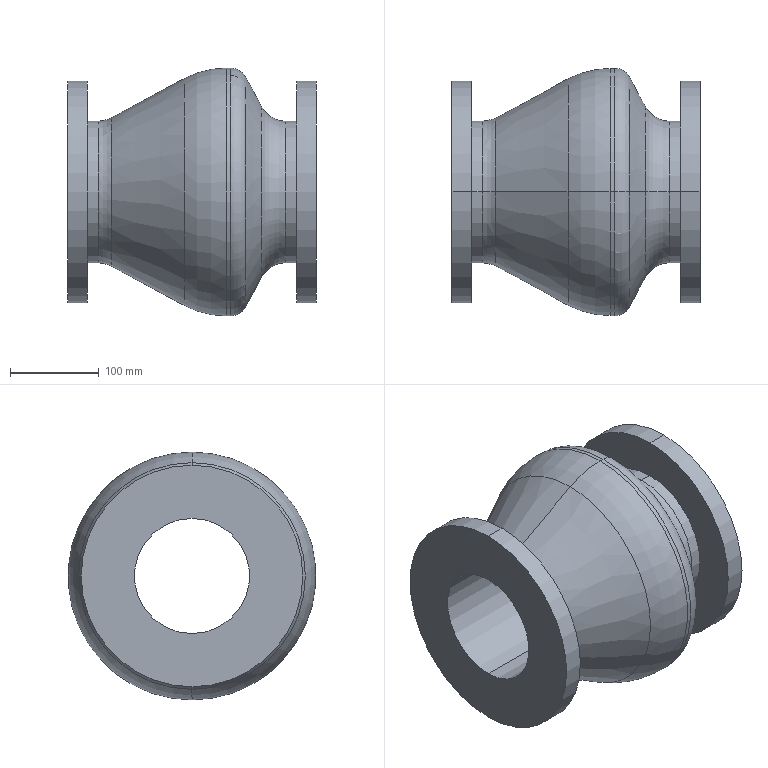Part | SolidWorks | features Revolution 1 | 1 solid | 28 faces | box 280 x 279.772 x 279.772 mm | volume 7581960 mm3 | cylinder 12 | torus 8 | cone 4 | plane 4 | commonest cylinder face diameters 160 x4 250 x4 130 x2 279.772 x2
STEP:
#1=CARTESIAN_POINT('',(34.398,0.,80.));
#2=VERTEX_POINT('',#1);
#3=CARTESIAN_POINT('',(34.398,0.,-80.));
#4=VERTEX_POINT('',#3);
#5=CARTESIAN_POINT('',(34.398,0.,0.));
#6=DIRECTION('',(-1.,0.,0.));
#7=DIRECTION('',(0.,0.,1.));
#8=AXIS2_PLACEMENT_3D('',#5,#6,#7);
#9=CIRCLE('',#8,80.);
#10=EDGE_CURVE('',#2,#4,#9,.T.);
#11=ORIENTED_EDGE('',*,*,#10,.T.);
#12=CARTESIAN_POINT('',(22.,0.,-80.));
#13=VERTEX_POINT('',#12);
#14=CARTESIAN_POINT('',(0.,0.,-80.));
#15=DIRECTION('',(-1.,0.,0.));
#16=VECTOR('',#15,1000.);
#17=LINE('',#14,#16);
#18=EDGE_CURVE('',#4,#13,#17,.T.);
#19=ORIENTED_EDGE('',*,*,#18,.T.);
#20=CARTESIAN_POINT('',(22.,0.,80.));
#21=VERTEX_POINT('',#20);
#22=CARTESIAN_POINT('',(22.,0.,0.));
#23=DIRECTION('',(-1.,0.,0.));
#24=DIRECTION('',(0.,0.,1.));
#25=AXIS2_PLACEMENT_3D('',#22,#23,#24);
#26=CIRCLE('',#25,80.);
#27=EDGE_CURVE('',#21,#13,#26,.T.);
#28=ORIENTED_EDGE('',*,*,#27,.F.);
#29=CARTESIAN_POINT('',(0.,0.,80.));
#30=DIRECTION('',(-1.,0.,0.));
#31=VECTOR('',#30,1000.);
#32=LINE('',#29,#31);
#33=EDGE_CURVE('',#2,#21,#32,.T.);
#34=ORIENTED_EDGE('',*,*,#33,.F.);
#35=EDGE_LOOP('',(#11,#19,#28,#34));
#36=FACE_OUTER_BOUND('',#35,.T.);
#37=CARTESIAN_POINT('',(0.,0.,0.));
#38=DIRECTION('',(-1.,0.,0.));
#39=DIRECTION('',(0.,0.,1.));
#40=AXIS2_PLACEMENT_3D('',#37,#38,#39);
#41=CYLINDRICAL_SURFACE('',#40,80.);
#42=ADVANCED_FACE('',(#36),#41,.T.);
#43=CARTESIAN_POINT('',(34.398,0.,0.));
#44=DIRECTION('',(-1.,0.,0.));
#45=DIRECTION('',(0.,0.,1.));
#46=AXIS2_PLACEMENT_3D('',#43,#44,#45);
#47=CIRCLE('',#46,80.);
#48=EDGE_CURVE('',#4,#2,#47,.T.);
#49=ORIENTED_EDGE('',*,*,#48,.F.);
#50=CARTESIAN_POINT('',(48.621,0.,-83.586));
#51=VERTEX_POINT('',#50);
#52=CARTESIAN_POINT('',(34.398,0.,-110.));
#53=DIRECTION('',(0.,1.,0.));
#54=DIRECTION('',(0.,0.,1.));
#55=AXIS2_PLACEMENT_3D('',#52,#53,#54);
#56=CIRCLE('',#55,30.);
#57=EDGE_CURVE('',#4,#51,#56,.T.);
#58=ORIENTED_EDGE('',*,*,#57,.T.);
#59=CARTESIAN_POINT('',(48.621,0.,83.586));
#60=VERTEX_POINT('',#59);
#61=CARTESIAN_POINT('',(48.621,0.,0.));
#62=DIRECTION('',(-1.,0.,0.));
#63=DIRECTION('',(0.,0.,1.));
#64=AXIS2_PLACEMENT_3D('',#61,#62,#63);
#65=CIRCLE('',#64,83.586);
#66=EDGE_CURVE('',#51,#60,#65,.T.);
#67=ORIENTED_EDGE('',*,*,#66,.T.);
#68=CARTESIAN_POINT('',(34.398,0.,110.));
#69=DIRECTION('',(0.,-1.,0.));
#70=DIRECTION('',(0.,0.,-1.));
#71=AXIS2_PLACEMENT_3D('',#68,#69,#70);
#72=CIRCLE('',#71,30.);
#73=EDGE_CURVE('',#2,#60,#72,.T.);
#74=ORIENTED_EDGE('',*,*,#73,.F.);
#75=EDGE_LOOP('',(#49,#58,#67,#74));
#76=FACE_OUTER_BOUND('',#75,.T.);
#77=CARTESIAN_POINT('',(34.398,0.,0.));
#78=DIRECTION('',(-1.,0.,0.));
#79=DIRECTION('',(0.,0.,1.));
#80=AXIS2_PLACEMENT_3D('',#77,#78,#79);
#81=TOROIDAL_SURFACE('',#80,110.,30.);
#82=ADVANCED_FACE('',(#76),#81,.F.);
#83=CARTESIAN_POINT('',(48.621,0.,0.));
#84=DIRECTION('',(-1.,0.,0.));
#85=DIRECTION('',(0.,0.,1.));
#86=AXIS2_PLACEMENT_3D('',#83,#84,#85);
#87=CIRCLE('',#86,83.586);
#88=EDGE_CURVE('',#60,#51,#87,.T.);
#89=ORIENTED_EDGE('',*,*,#88,.F.);
#90=CARTESIAN_POINT('',(130.98,0.,127.933));
#91=VERTEX_POINT('',#90);
#92=CARTESIAN_POINT('',(130.98,0.,127.933));
#93=DIRECTION('',(0.8805,0.,0.4741));
#94=VECTOR('',#93,1000.);
#95=LINE('',#92,#94);
#96=EDGE_CURVE('',#60,#91,#95,.T.);
#97=ORIENTED_EDGE('',*,*,#96,.T.);
#98=CARTESIAN_POINT('',(130.98,0.,-127.933));
#99=VERTEX_POINT('',#98);
#100=CARTESIAN_POINT('',(130.98,0.,0.));
#101=DIRECTION('',(-1.,0.,0.));
#102=DIRECTION('',(0.,0.,1.));
#103=AXIS2_PLACEMENT_3D('',#100,#101,#102);
#104=CIRCLE('',#103,127.933);
#105=EDGE_CURVE('',#91,#99,#104,.T.);
#106=ORIENTED_EDGE('',*,*,#105,.T.);
#107=CARTESIAN_POINT('',(130.98,0.,-127.933));
#108=DIRECTION('',(0.8805,0.,-0.4741));
#109=VECTOR('',#108,1000.);
#110=LINE('',#107,#109);
#111=EDGE_CURVE('',#51,#99,#110,.T.);
#112=ORIENTED_EDGE('',*,*,#111,.F.);
#113=EDGE_LOOP('',(#89,#97,#106,#112));
#114=FACE_OUTER_BOUND('',#113,.T.);
#115=CARTESIAN_POINT('',(130.98,0.,0.));
#116=DIRECTION('',(1.,0.,0.));
#117=DIRECTION('',(0.,0.,-1.));
#118=AXIS2_PLACEMENT_3D('',#115,#116,#117);
#119=CONICAL_SURFACE('',#118,127.933,0.4939);
#120=ADVANCED_FACE('',(#114),#119,.T.);
#121=CARTESIAN_POINT('',(178.39,0.,139.886));
#122=VERTEX_POINT('',#121);
#123=CARTESIAN_POINT('',(178.39,0.,-139.886));
#124=VERTEX_POINT('',#123);
#125=CARTESIAN_POINT('',(178.39,0.,0.));
#126=DIRECTION('',(-1.,0.,0.));
#127=DIRECTION('',(0.,0.,1.));
#128=AXIS2_PLACEMENT_3D('',#125,#126,#127);
#129=CIRCLE('',#128,139.886);
#130=EDGE_CURVE('',#122,#124,#129,.T.);
#131=ORIENTED_EDGE('',*,*,#130,.T.);
#132=CARTESIAN_POINT('',(178.39,0.,-39.886));
#133=DIRECTION('',(0.,1.,0.));
#134=DIRECTION('',(0.,0.,1.));
#135=AXIS2_PLACEMENT_3D('',#132,#133,#134);
#136=CIRCLE('',#135,100.);
#137=EDGE_CURVE('',#124,#99,#136,.T.);
#138=ORIENTED_EDGE('',*,*,#137,.T.);
#139=ORIENTED_EDGE('',*,*,#105,.F.);
#140=CARTESIAN_POINT('',(178.39,0.,39.886));
#141=DIRECTION('',(0.,-1.,0.));
#142=DIRECTION('',(0.,0.,-1.));
#143=AXIS2_PLACEMENT_3D('',#140,#141,#142);
#144=CIRCLE('',#143,100.);
#145=EDGE_CURVE('',#122,#91,#144,.T.);
#146=ORIENTED_EDGE('',*,*,#145,.F.);
#147=EDGE_LOOP('',(#131,#138,#139,#146));
#148=FACE_OUTER_BOUND('',#147,.T.);
#149=CARTESIAN_POINT('',(178.39,0.,0.));
#150=DIRECTION('',(-1.,0.,0.));
#151=DIRECTION('',(0.,0.,1.));
#152=AXIS2_PLACEMENT_3D('',#149,#150,#151);
#153=TOROIDAL_SURFACE('',#152,39.886,100.);
#154=ADVANCED_FACE('',(#148),#153,.T.);
#155=CARTESIAN_POINT('',(183.058,0.,139.886));
#156=VERTEX_POINT('',#155);
#157=CARTESIAN_POINT('',(183.058,0.,-139.886));
#158=VERTEX_POINT('',#157);
#159=CARTESIAN_POINT('',(183.058,0.,0.));
#160=DIRECTION('',(-1.,0.,0.));
#161=DIRECTION('',(0.,0.,1.));
#162=AXIS2_PLACEMENT_3D('',#159,#160,#161);
#163=CIRCLE('',#162,139.886);
#164=EDGE_CURVE('',#156,#158,#163,.T.);
#165=ORIENTED_EDGE('',*,*,#164,.T.);
#166=CARTESIAN_POINT('',(0.,0.,-139.886));
#167=DIRECTION('',(-1.,0.,0.));
#168=VECTOR('',#167,1000.);
#169=LINE('',#166,#168);
#170=EDGE_CURVE('',#158,#124,#169,.T.);
#171=ORIENTED_EDGE('',*,*,#170,.T.);
#172=ORIENTED_EDGE('',*,*,#130,.F.);
#173=CARTESIAN_POINT('',(0.,0.,139.886));
#174=DIRECTION('',(-1.,0.,0.));
#175=VECTOR('',#174,1000.);
#176=LINE('',#173,#175);
#177=EDGE_CURVE('',#156,#122,#176,.T.);
#178=ORIENTED_EDGE('',*,*,#177,.F.);
#179=EDGE_LOOP('',(#165,#171,#172,#178));
#180=FACE_OUTER_BOUND('',#179,.T.);
#181=CARTESIAN_POINT('',(0.,0.,0.));
#182=DIRECTION('',(-1.,0.,0.));
#183=DIRECTION('',(0.,0.,1.));
#184=AXIS2_PLACEMENT_3D('',#181,#182,#183);
#185=CYLINDRICAL_SURFACE('',#184,139.886);
#186=ADVANCED_FACE('',(#180),#185,.T.);
#187=CARTESIAN_POINT('',(200.667,0.,129.368));
#188=VERTEX_POINT('',#187);
#189=CARTESIAN_POINT('',(200.667,0.,-129.368));
#190=VERTEX_POINT('',#189);
#191=CARTESIAN_POINT('',(200.667,0.,0.));
#192=DIRECTION('',(-1.,0.,0.));
#193=DIRECTION('',(0.,0.,1.));
#194=AXIS2_PLACEMENT_3D('',#191,#192,#193);
#195=CIRCLE('',#194,129.368);
#196=EDGE_CURVE('',#188,#190,#195,.T.);
#197=ORIENTED_EDGE('',*,*,#196,.T.);
#198=CARTESIAN_POINT('',(183.058,0.,-119.886));
#199=DIRECTION('',(0.,1.,0.));
#200=DIRECTION('',(0.,0.,1.));
#201=AXIS2_PLACEMENT_3D('',#198,#199,#200);
#202=CIRCLE('',#201,20.);
#203=EDGE_CURVE('',#190,#158,#202,.T.);
#204=ORIENTED_EDGE('',*,*,#203,.T.);
#205=ORIENTED_EDGE('',*,*,#164,.F.);
#206=CARTESIAN_POINT('',(183.058,0.,119.886));
#207=DIRECTION('',(0.,-1.,0.));
#208=DIRECTION('',(0.,0.,-1.));
#209=AXIS2_PLACEMENT_3D('',#206,#207,#208);
#210=CIRCLE('',#209,20.);
#211=EDGE_CURVE('',#188,#156,#210,.T.);
#212=ORIENTED_EDGE('',*,*,#211,.F.);
#213=EDGE_LOOP('',(#197,#204,#205,#212));
#214=FACE_OUTER_BOUND('',#213,.T.);
#215=CARTESIAN_POINT('',(183.058,0.,0.));
#216=DIRECTION('',(-1.,0.,0.));
#217=DIRECTION('',(0.,0.,1.));
#218=AXIS2_PLACEMENT_3D('',#215,#216,#217);
#219=TOROIDAL_SURFACE('',#218,119.886,20.);
#220=ADVANCED_FACE('',(#214),#219,.T.);
#221=CARTESIAN_POINT('',(218.755,0.,95.777));
#222=VERTEX_POINT('',#221);
#223=CARTESIAN_POINT('',(218.755,0.,-95.777));
#224=VERTEX_POINT('',#223);
#225=CARTESIAN_POINT('',(218.755,0.,0.));
#226=DIRECTION('',(-1.,0.,0.));
#227=DIRECTION('',(0.,0.,1.));
#228=AXIS2_PLACEMENT_3D('',#225,#226,#227);
#229=CIRCLE('',#228,95.777);
#230=EDGE_CURVE('',#222,#224,#229,.T.);
#231=ORIENTED_EDGE('',*,*,#230,.T.);
#232=CARTESIAN_POINT('',(218.755,0.,-95.777));
#233=DIRECTION('',(-0.4741,0.,-0.8805));
#234=VECTOR('',#233,1000.);
#235=LINE('',#232,#234);
#236=EDGE_CURVE('',#224,#190,#235,.T.);
#237=ORIENTED_EDGE('',*,*,#236,.T.);
#238=ORIENTED_EDGE('',*,*,#196,.F.);
#239=CARTESIAN_POINT('',(218.755,0.,95.777));
#240=DIRECTION('',(-0.4741,0.,0.8805));
#241=VECTOR('',#240,1000.);
#242=LINE('',#239,#241);
#243=EDGE_CURVE('',#222,#188,#242,.T.);
#244=ORIENTED_EDGE('',*,*,#243,.F.);
#245=EDGE_LOOP('',(#231,#237,#238,#244));
#246=FACE_OUTER_BOUND('',#245,.T.);
#247=CARTESIAN_POINT('',(218.755,0.,0.));
#248=DIRECTION('',(-1.,0.,0.));
#249=DIRECTION('',(0.,0.,1.));
#250=AXIS2_PLACEMENT_3D('',#247,#248,#249);
#251=CONICAL_SURFACE('',#250,95.777,1.077);
#252=ADVANCED_FACE('',(#246),#251,.T.);
#253=CARTESIAN_POINT('',(218.755,0.,0.));
#254=DIRECTION('',(-1.,0.,0.));
#255=DIRECTION('',(0.,0.,1.));
#256=AXIS2_PLACEMENT_3D('',#253,#254,#255);
#257=CIRCLE('',#256,95.777);
#258=EDGE_CURVE('',#224,#222,#257,.T.);
#259=ORIENTED_EDGE('',*,*,#258,.F.);
#260=CARTESIAN_POINT('',(245.169,0.,-80.));
#261=VERTEX_POINT('',#260);
#262=CARTESIAN_POINT('',(245.169,0.,-110.));
#263=DIRECTION('',(0.,1.,0.));
#264=DIRECTION('',(0.,0.,1.));
#265=AXIS2_PLACEMENT_3D('',#262,#263,#264);
#266=CIRCLE('',#265,30.);
#267=EDGE_CURVE('',#224,#261,#266,.T.);
#268=ORIENTED_EDGE('',*,*,#267,.T.);
#269=CARTESIAN_POINT('',(245.169,0.,80.));
#270=VERTEX_POINT('',#269);
#271=CARTESIAN_POINT('',(245.169,0.,0.));
#272=DIRECTION('',(-1.,0.,0.));
#273=DIRECTION('',(0.,0.,1.));
#274=AXIS2_PLACEMENT_3D('',#271,#272,#273);
#275=CIRCLE('',#274,80.);
#276=EDGE_CURVE('',#261,#270,#275,.T.);
#277=ORIENTED_EDGE('',*,*,#276,.T.);
#278=CARTESIAN_POINT('',(245.169,0.,110.));
#279=DIRECTION('',(0.,-1.,0.));
#280=DIRECTION('',(0.,0.,-1.));
#281=AXIS2_PLACEMENT_3D('',#278,#279,#280);
#282=CIRCLE('',#281,30.);
#283=EDGE_CURVE('',#222,#270,#282,.T.);
#284=ORIENTED_EDGE('',*,*,#283,.F.);
#285=EDGE_LOOP('',(#259,#268,#277,#284));
#286=FACE_OUTER_BOUND('',#285,.T.);
#287=CARTESIAN_POINT('',(245.169,0.,0.));
#288=DIRECTION('',(-1.,0.,0.));
#289=DIRECTION('',(0.,0.,1.));
#290=AXIS2_PLACEMENT_3D('',#287,#288,#289);
#291=TOROIDAL_SURFACE('',#290,110.,30.);
#292=ADVANCED_FACE('',(#286),#291,.F.);
#293=CARTESIAN_POINT('',(258.,0.,80.));
#294=VERTEX_POINT('',#293);
#295=CARTESIAN_POINT('',(258.,0.,-80.));
#296=VERTEX_POINT('',#295);
#297=CARTESIAN_POINT('',(258.,0.,0.));
#298=DIRECTION('',(-1.,0.,0.));
#299=DIRECTION('',(0.,0.,1.));
#300=AXIS2_PLACEMENT_3D('',#297,#298,#299);
#301=CIRCLE('',#300,80.);
#302=EDGE_CURVE('',#294,#296,#301,.T.);
#303=ORIENTED_EDGE('',*,*,#302,.T.);
#304=CARTESIAN_POINT('',(0.,0.,-80.));
#305=DIRECTION('',(-1.,0.,0.));
#306=VECTOR('',#305,1000.);
#307=LINE('',#304,#306);
#308=EDGE_CURVE('',#296,#261,#307,.T.);
#309=ORIENTED_EDGE('',*,*,#308,.T.);
#310=CARTESIAN_POINT('',(245.169,0.,0.));
#311=DIRECTION('',(-1.,0.,0.));
#312=DIRECTION('',(0.,0.,1.));
#313=AXIS2_PLACEMENT_3D('',#310,#311,#312);
#314=CIRCLE('',#313,80.);
#315=EDGE_CURVE('',#270,#261,#314,.T.);
#316=ORIENTED_EDGE('',*,*,#315,.F.);
#317=CARTESIAN_POINT('',(0.,0.,80.));
#318=DIRECTION('',(-1.,0.,0.));
#319=VECTOR('',#318,1000.);
#320=LINE('',#317,#319);
#321=EDGE_CURVE('',#294,#270,#320,.T.);
#322=ORIENTED_EDGE('',*,*,#321,.F.);
#323=EDGE_LOOP('',(#303,#309,#316,#322));
#324=FACE_OUTER_BOUND('',#323,.T.);
#325=CARTESIAN_POINT('',(0.,0.,0.));
#326=DIRECTION('',(-1.,0.,0.));
#327=DIRECTION('',(0.,0.,1.));
#328=AXIS2_PLACEMENT_3D('',#325,#326,#327);
#329=CYLINDRICAL_SURFACE('',#328,80.);
#330=ADVANCED_FACE('',(#324),#329,.T.);
#331=CARTESIAN_POINT('',(280.,0.,125.));
#332=VERTEX_POINT('',#331);
#333=CARTESIAN_POINT('',(280.,0.,-125.));
#334=VERTEX_POINT('',#333);
#335=CARTESIAN_POINT('',(280.,0.,0.));
#336=DIRECTION('',(-1.,0.,0.));
#337=DIRECTION('',(0.,0.,1.));
#338=AXIS2_PLACEMENT_3D('',#335,#336,#337);
#339=CIRCLE('',#338,125.);
#340=EDGE_CURVE('',#332,#334,#339,.T.);
#341=ORIENTED_EDGE('',*,*,#340,.T.);
#342=CARTESIAN_POINT('',(258.,0.,-125.));
#343=VERTEX_POINT('',#342);
#344=CARTESIAN_POINT('',(0.,0.,-125.));
#345=DIRECTION('',(-1.,0.,0.));
#346=VECTOR('',#345,1000.);
#347=LINE('',#344,#346);
#348=EDGE_CURVE('',#334,#343,#347,.T.);
#349=ORIENTED_EDGE('',*,*,#348,.T.);
#350=CARTESIAN_POINT('',(258.,0.,125.));
#351=VERTEX_POINT('',#350);
#352=CARTESIAN_POINT('',(258.,0.,0.));
#353=DIRECTION('',(-1.,0.,0.));
#354=DIRECTION('',(0.,0.,1.));
#355=AXIS2_PLACEMENT_3D('',#352,#353,#354);
#356=CIRCLE('',#355,125.);
#357=EDGE_CURVE('',#351,#343,#356,.T.);
#358=ORIENTED_EDGE('',*,*,#357,.F.);
#359=CARTESIAN_POINT('',(0.,0.,125.));
#360=DIRECTION('',(-1.,0.,0.));
#361=VECTOR('',#360,1000.);
#362=LINE('',#359,#361);
#363=EDGE_CURVE('',#332,#351,#362,.T.);
#364=ORIENTED_EDGE('',*,*,#363,.F.);
#365=EDGE_LOOP('',(#341,#349,#358,#364));
#366=FACE_OUTER_BOUND('',#365,.T.);
#367=CARTESIAN_POINT('',(0.,0.,0.));
#368=DIRECTION('',(-1.,0.,0.));
#369=DIRECTION('',(0.,0.,1.));
#370=AXIS2_PLACEMENT_3D('',#367,#368,#369);
#371=CYLINDRICAL_SURFACE('',#370,125.);
#372=ADVANCED_FACE('',(#366),#371,.T.);
#373=CARTESIAN_POINT('',(280.,0.,-65.));
#374=VERTEX_POINT('',#373);
#375=CARTESIAN_POINT('',(280.,0.,65.));
#376=VERTEX_POINT('',#375);
#377=CARTESIAN_POINT('',(280.,0.,0.));
#378=DIRECTION('',(-1.,0.,0.));
#379=DIRECTION('',(0.,0.,1.));
#380=AXIS2_PLACEMENT_3D('',#377,#378,#379);
#381=CIRCLE('',#380,65.);
#382=EDGE_CURVE('',#374,#376,#381,.T.);
#383=ORIENTED_EDGE('',*,*,#382,.F.);
#384=CARTESIAN_POINT('',(0.,0.,-65.));
#385=VERTEX_POINT('',#384);
#386=CARTESIAN_POINT('',(0.,0.,-65.));
#387=DIRECTION('',(-1.,0.,0.));
#388=VECTOR('',#387,1000.);
#389=LINE('',#386,#388);
#390=EDGE_CURVE('',#374,#385,#389,.T.);
#391=ORIENTED_EDGE('',*,*,#390,.T.);
#392=CARTESIAN_POINT('',(0.,0.,65.));
#393=VERTEX_POINT('',#392);
#394=CARTESIAN_POINT('',(0.,0.,0.));
#395=DIRECTION('',(-1.,0.,0.));
#396=DIRECTION('',(0.,0.,1.));
#397=AXIS2_PLACEMENT_3D('',#394,#395,#396);
#398=CIRCLE('',#397,65.);
#399=EDGE_CURVE('',#385,#393,#398,.T.);
#400=ORIENTED_EDGE('',*,*,#399,.T.);
#401=CARTESIAN_POINT('',(0.,0.,65.));
#402=DIRECTION('',(-1.,0.,0.));
#403=VECTOR('',#402,1000.);
#404=LINE('',#401,#403);
#405=EDGE_CURVE('',#376,#393,#404,.T.);
#406=ORIENTED_EDGE('',*,*,#405,.F.);
#407=EDGE_LOOP('',(#383,#391,#400,#406));
#408=FACE_OUTER_BOUND('',#407,.T.);
#409=CARTESIAN_POINT('',(0.,0.,0.));
#410=DIRECTION('',(-1.,0.,0.));
#411=DIRECTION('',(0.,0.,1.));
#412=AXIS2_PLACEMENT_3D('',#409,#410,#411);
#413=CYLINDRICAL_SURFACE('',#412,65.);
#414=ADVANCED_FACE('',(#408),#413,.F.);
#415=CARTESIAN_POINT('',(22.,0.,125.));
#416=VERTEX_POINT('',#415);
#417=CARTESIAN_POINT('',(22.,0.,-125.));
#418=VERTEX_POINT('',#417);
#419=CARTESIAN_POINT('',(22.,0.,0.));
#420=DIRECTION('',(-1.,0.,0.));
#421=DIRECTION('',(0.,0.,1.));
#422=AXIS2_PLACEMENT_3D('',#419,#420,#421);
#423=CIRCLE('',#422,125.);
#424=EDGE_CURVE('',#416,#418,#423,.T.);
#425=ORIENTED_EDGE('',*,*,#424,.T.);
#426=CARTESIAN_POINT('',(0.,0.,-125.));
#427=VERTEX_POINT('',#426);
#428=CARTESIAN_POINT('',(0.,0.,-125.));
#429=DIRECTION('',(-1.,0.,0.));
#430=VECTOR('',#429,1000.);
#431=LINE('',#428,#430);
#432=EDGE_CURVE('',#418,#427,#431,.T.);
#433=ORIENTED_EDGE('',*,*,#432,.T.);
#434=CARTESIAN_POINT('',(0.,0.,125.));
#435=VERTEX_POINT('',#434);
#436=CARTESIAN_POINT('',(0.,0.,0.));
#437=DIRECTION('',(-1.,0.,0.));
#438=DIRECTION('',(0.,0.,1.));
#439=AXIS2_PLACEMENT_3D('',#436,#437,#438);
#440=CIRCLE('',#439,125.);
#441=EDGE_CURVE('',#435,#427,#440,.T.);
#442=ORIENTED_EDGE('',*,*,#441,.F.);
#443=CARTESIAN_POINT('',(0.,0.,125.));
#444=DIRECTION('',(-1.,0.,0.));
#445=VECTOR('',#444,1000.);
#446=LINE('',#443,#445);
#447=EDGE_CURVE('',#416,#435,#446,.T.);
#448=ORIENTED_EDGE('',*,*,#447,.F.);
#449=EDGE_LOOP('',(#425,#433,#442,#448));
#450=FACE_OUTER_BOUND('',#449,.T.);
#451=CARTESIAN_POINT('',(0.,0.,0.));
#452=DIRECTION('',(-1.,0.,0.));
#453=DIRECTION('',(0.,0.,1.));
#454=AXIS2_PLACEMENT_3D('',#451,#452,#453);
#455=CYLINDRICAL_SURFACE('',#454,125.);
#456=ADVANCED_FACE('',(#450),#455,.T.);
#457=ORIENTED_EDGE('',*,*,#432,.F.);
#458=CARTESIAN_POINT('',(22.,0.,0.));
#459=DIRECTION('',(-1.,0.,0.));
#460=DIRECTION('',(0.,0.,1.));
#461=AXIS2_PLACEMENT_3D('',#458,#459,#460);
#462=CIRCLE('',#461,125.);
#463=EDGE_CURVE('',#418,#416,#462,.T.);
#464=ORIENTED_EDGE('',*,*,#463,.T.);
#465=ORIENTED_EDGE('',*,*,#447,.T.);
#466=CARTESIAN_POINT('',(0.,0.,0.));
#467=DIRECTION('',(-1.,0.,0.));
#468=DIRECTION('',(0.,0.,1.));
#469=AXIS2_PLACEMENT_3D('',#466,#467,#468);
#470=CIRCLE('',#469,125.);
#471=EDGE_CURVE('',#427,#435,#470,.T.);
#472=ORIENTED_EDGE('',*,*,#471,.F.);
#473=EDGE_LOOP('',(#457,#464,#465,#472));
#474=FACE_OUTER_BOUND('',#473,.T.);
#475=CARTESIAN_POINT('',(0.,0.,0.));
#476=DIRECTION('',(-1.,0.,0.));
#477=DIRECTION('',(0.,0.,1.));
#478=AXIS2_PLACEMENT_3D('',#475,#476,#477);
#479=CYLINDRICAL_SURFACE('',#478,125.);
#480=ADVANCED_FACE('',(#474),#479,.T.);
#481=CARTESIAN_POINT('',(0.,0.,0.));
#482=DIRECTION('',(-1.,0.,0.));
#483=DIRECTION('',(0.,0.,1.));
#484=AXIS2_PLACEMENT_3D('',#481,#482,#483);
#485=CIRCLE('',#484,65.);
#486=EDGE_CURVE('',#393,#385,#485,.T.);
#487=ORIENTED_EDGE('',*,*,#486,.F.);
#488=ORIENTED_EDGE('',*,*,#399,.F.);
#489=EDGE_LOOP('',(#487,#488));
#490=FACE_BOUND('',#489,.T.);
#491=ORIENTED_EDGE('',*,*,#441,.T.);
#492=ORIENTED_EDGE('',*,*,#471,.T.);
#493=EDGE_LOOP('',(#491,#492));
#494=FACE_OUTER_BOUND('',#493,.T.);
#495=CARTESIAN_POINT('',(0.,65.,0.));
#496=DIRECTION('',(1.,0.,0.));
#497=DIRECTION('',(0.,0.,-1.));
#498=AXIS2_PLACEMENT_3D('',#495,#496,#497);
#499=PLANE('',#498);
#500=ADVANCED_FACE('',(#490,#494),#499,.F.);
#501=ORIENTED_EDGE('',*,*,#390,.F.);
#502=CARTESIAN_POINT('',(280.,0.,0.));
#503=DIRECTION('',(-1.,0.,0.));
#504=DIRECTION('',(0.,0.,1.));
#505=AXIS2_PLACEMENT_3D('',#502,#503,#504);
#506=CIRCLE('',#505,65.);
#507=EDGE_CURVE('',#376,#374,#506,.T.);
#508=ORIENTED_EDGE('',*,*,#507,.F.);
#509=ORIENTED_EDGE('',*,*,#405,.T.);
#510=ORIENTED_EDGE('',*,*,#486,.T.);
#511=EDGE_LOOP('',(#501,#508,#509,#510));
#512=FACE_OUTER_BOUND('',#511,.T.);
#513=CARTESIAN_POINT('',(0.,0.,0.));
#514=DIRECTION('',(-1.,0.,0.));
#515=DIRECTION('',(0.,0.,1.));
#516=AXIS2_PLACEMENT_3D('',#513,#514,#515);
#517=CYLINDRICAL_SURFACE('',#516,65.);
#518=ADVANCED_FACE('',(#512),#517,.F.);
#519=ORIENTED_EDGE('',*,*,#340,.F.);
#520=CARTESIAN_POINT('',(280.,0.,0.));
#521=DIRECTION('',(-1.,0.,0.));
#522=DIRECTION('',(0.,0.,1.));
#523=AXIS2_PLACEMENT_3D('',#520,#521,#522);
#524=CIRCLE('',#523,125.);
#525=EDGE_CURVE('',#334,#332,#524,.T.);
#526=ORIENTED_EDGE('',*,*,#525,.F.);
#527=EDGE_LOOP('',(#519,#526));
#528=FACE_OUTER_BOUND('',#527,.T.);
#529=ORIENTED_EDGE('',*,*,#507,.T.);
#530=ORIENTED_EDGE('',*,*,#382,.T.);
#531=EDGE_LOOP('',(#529,#530));
#532=FACE_BOUND('',#531,.T.);
#533=CARTESIAN_POINT('',(280.,125.,0.));
#534=DIRECTION('',(-1.,0.,0.));
#535=DIRECTION('',(0.,0.,1.));
#536=AXIS2_PLACEMENT_3D('',#533,#534,#535);
#537=PLANE('',#536);
#538=ADVANCED_FACE('',(#528,#532),#537,.F.);
#539=ORIENTED_EDGE('',*,*,#348,.F.);
#540=ORIENTED_EDGE('',*,*,#525,.T.);
#541=ORIENTED_EDGE('',*,*,#363,.T.);
#542=CARTESIAN_POINT('',(258.,0.,0.));
#543=DIRECTION('',(-1.,0.,0.));
#544=DIRECTION('',(0.,0.,1.));
#545=AXIS2_PLACEMENT_3D('',#542,#543,#544);
#546=CIRCLE('',#545,125.);
#547=EDGE_CURVE('',#343,#351,#546,.T.);
#548=ORIENTED_EDGE('',*,*,#547,.F.);
#549=EDGE_LOOP('',(#539,#540,#541,#548));
#550=FACE_OUTER_BOUND('',#549,.T.);
#551=CARTESIAN_POINT('',(0.,0.,0.));
#552=DIRECTION('',(-1.,0.,0.));
#553=DIRECTION('',(0.,0.,1.));
#554=AXIS2_PLACEMENT_3D('',#551,#552,#553);
#555=CYLINDRICAL_SURFACE('',#554,125.);
#556=ADVANCED_FACE('',(#550),#555,.T.);
#557=ORIENTED_EDGE('',*,*,#302,.F.);
#558=CARTESIAN_POINT('',(258.,0.,0.));
#559=DIRECTION('',(-1.,0.,0.));
#560=DIRECTION('',(0.,0.,1.));
#561=AXIS2_PLACEMENT_3D('',#558,#559,#560);
#562=CIRCLE('',#561,80.);
#563=EDGE_CURVE('',#296,#294,#562,.T.);
#564=ORIENTED_EDGE('',*,*,#563,.F.);
#565=EDGE_LOOP('',(#557,#564));
#566=FACE_BOUND('',#565,.T.);
#567=ORIENTED_EDGE('',*,*,#357,.T.);
#568=ORIENTED_EDGE('',*,*,#547,.T.);
#569=EDGE_LOOP('',(#567,#568));
#570=FACE_OUTER_BOUND('',#569,.T.);
#571=CARTESIAN_POINT('',(258.,80.,0.));
#572=DIRECTION('',(1.,0.,0.));
#573=DIRECTION('',(0.,0.,-1.));
#574=AXIS2_PLACEMENT_3D('',#571,#572,#573);
#575=PLANE('',#574);
#576=ADVANCED_FACE('',(#566,#570),#575,.F.);
#577=ORIENTED_EDGE('',*,*,#308,.F.);
#578=ORIENTED_EDGE('',*,*,#563,.T.);
#579=ORIENTED_EDGE('',*,*,#321,.T.);
#580=ORIENTED_EDGE('',*,*,#276,.F.);
#581=EDGE_LOOP('',(#577,#578,#579,#580));
#582=FACE_OUTER_BOUND('',#581,.T.);
#583=CARTESIAN_POINT('',(0.,0.,0.));
#584=DIRECTION('',(-1.,0.,0.));
#585=DIRECTION('',(0.,0.,1.));
#586=AXIS2_PLACEMENT_3D('',#583,#584,#585);
#587=CYLINDRICAL_SURFACE('',#586,80.);
#588=ADVANCED_FACE('',(#582),#587,.T.);
#589=ORIENTED_EDGE('',*,*,#267,.F.);
#590=ORIENTED_EDGE('',*,*,#230,.F.);
#591=ORIENTED_EDGE('',*,*,#283,.T.);
#592=ORIENTED_EDGE('',*,*,#315,.T.);
#593=EDGE_LOOP('',(#589,#590,#591,#592));
#594=FACE_OUTER_BOUND('',#593,.T.);
#595=CARTESIAN_POINT('',(245.169,0.,0.));
#596=DIRECTION('',(-1.,0.,0.));
#597=DIRECTION('',(0.,0.,1.));
#598=AXIS2_PLACEMENT_3D('',#595,#596,#597);
#599=TOROIDAL_SURFACE('',#598,110.,30.);
#600=ADVANCED_FACE('',(#594),#599,.F.);
#601=ORIENTED_EDGE('',*,*,#236,.F.);
#602=ORIENTED_EDGE('',*,*,#258,.T.);
#603=ORIENTED_EDGE('',*,*,#243,.T.);
#604=CARTESIAN_POINT('',(200.667,0.,0.));
#605=DIRECTION('',(-1.,0.,0.));
#606=DIRECTION('',(0.,0.,1.));
#607=AXIS2_PLACEMENT_3D('',#604,#605,#606);
#608=CIRCLE('',#607,129.368);
#609=EDGE_CURVE('',#190,#188,#608,.T.);
#610=ORIENTED_EDGE('',*,*,#609,.F.);
#611=EDGE_LOOP('',(#601,#602,#603,#610));
#612=FACE_OUTER_BOUND('',#611,.T.);
#613=CARTESIAN_POINT('',(218.755,0.,0.));
#614=DIRECTION('',(-1.,0.,0.));
#615=DIRECTION('',(0.,0.,1.));
#616=AXIS2_PLACEMENT_3D('',#613,#614,#615);
#617=CONICAL_SURFACE('',#616,95.777,1.077);
#618=ADVANCED_FACE('',(#612),#617,.T.);
#619=ORIENTED_EDGE('',*,*,#203,.F.);
#620=ORIENTED_EDGE('',*,*,#609,.T.);
#621=ORIENTED_EDGE('',*,*,#211,.T.);
#622=CARTESIAN_POINT('',(183.058,0.,0.));
#623=DIRECTION('',(-1.,0.,0.));
#624=DIRECTION('',(0.,0.,1.));
#625=AXIS2_PLACEMENT_3D('',#622,#623,#624);
#626=CIRCLE('',#625,139.886);
#627=EDGE_CURVE('',#158,#156,#626,.T.);
#628=ORIENTED_EDGE('',*,*,#627,.F.);
#629=EDGE_LOOP('',(#619,#620,#621,#628));
#630=FACE_OUTER_BOUND('',#629,.T.);
#631=CARTESIAN_POINT('',(183.058,0.,0.));
#632=DIRECTION('',(-1.,0.,0.));
#633=DIRECTION('',(0.,0.,1.));
#634=AXIS2_PLACEMENT_3D('',#631,#632,#633);
#635=TOROIDAL_SURFACE('',#634,119.886,20.);
#636=ADVANCED_FACE('',(#630),#635,.T.);
#637=ORIENTED_EDGE('',*,*,#170,.F.);
#638=ORIENTED_EDGE('',*,*,#627,.T.);
#639=ORIENTED_EDGE('',*,*,#177,.T.);
#640=CARTESIAN_POINT('',(178.39,0.,0.));
#641=DIRECTION('',(-1.,0.,0.));
#642=DIRECTION('',(0.,0.,1.));
#643=AXIS2_PLACEMENT_3D('',#640,#641,#642);
#644=CIRCLE('',#643,139.886);
#645=EDGE_CURVE('',#124,#122,#644,.T.);
#646=ORIENTED_EDGE('',*,*,#645,.F.);
#647=EDGE_LOOP('',(#637,#638,#639,#646));
#648=FACE_OUTER_BOUND('',#647,.T.);
#649=CARTESIAN_POINT('',(0.,0.,0.));
#650=DIRECTION('',(-1.,0.,0.));
#651=DIRECTION('',(0.,0.,1.));
#652=AXIS2_PLACEMENT_3D('',#649,#650,#651);
#653=CYLINDRICAL_SURFACE('',#652,139.886);
#654=ADVANCED_FACE('',(#648),#653,.T.);
#655=ORIENTED_EDGE('',*,*,#137,.F.);
#656=ORIENTED_EDGE('',*,*,#645,.T.);
#657=ORIENTED_EDGE('',*,*,#145,.T.);
#658=CARTESIAN_POINT('',(130.98,0.,0.));
#659=DIRECTION('',(-1.,0.,0.));
#660=DIRECTION('',(0.,0.,1.));
#661=AXIS2_PLACEMENT_3D('',#658,#659,#660);
#662=CIRCLE('',#661,127.933);
#663=EDGE_CURVE('',#99,#91,#662,.T.);
#664=ORIENTED_EDGE('',*,*,#663,.F.);
#665=EDGE_LOOP('',(#655,#656,#657,#664));
#666=FACE_OUTER_BOUND('',#665,.T.);
#667=CARTESIAN_POINT('',(178.39,0.,0.));
#668=DIRECTION('',(-1.,0.,0.));
#669=DIRECTION('',(0.,0.,1.));
#670=AXIS2_PLACEMENT_3D('',#667,#668,#669);
#671=TOROIDAL_SURFACE('',#670,39.886,100.);
#672=ADVANCED_FACE('',(#666),#671,.T.);
#673=ORIENTED_EDGE('',*,*,#96,.F.);
#674=ORIENTED_EDGE('',*,*,#66,.F.);
#675=ORIENTED_EDGE('',*,*,#111,.T.);
#676=ORIENTED_EDGE('',*,*,#663,.T.);
#677=EDGE_LOOP('',(#673,#674,#675,#676));
#678=FACE_OUTER_BOUND('',#677,.T.);
#679=CARTESIAN_POINT('',(130.98,0.,0.));
#680=DIRECTION('',(1.,0.,0.));
#681=DIRECTION('',(0.,0.,-1.));
#682=AXIS2_PLACEMENT_3D('',#679,#680,#681);
#683=CONICAL_SURFACE('',#682,127.933,0.4939);
#684=ADVANCED_FACE('',(#678),#683,.T.);
#685=ORIENTED_EDGE('',*,*,#57,.F.);
#686=ORIENTED_EDGE('',*,*,#10,.F.);
#687=ORIENTED_EDGE('',*,*,#73,.T.);
#688=ORIENTED_EDGE('',*,*,#88,.T.);
#689=EDGE_LOOP('',(#685,#686,#687,#688));
#690=FACE_OUTER_BOUND('',#689,.T.);
#691=CARTESIAN_POINT('',(34.398,0.,0.));
#692=DIRECTION('',(-1.,0.,0.));
#693=DIRECTION('',(0.,0.,1.));
#694=AXIS2_PLACEMENT_3D('',#691,#692,#693);
#695=TOROIDAL_SURFACE('',#694,110.,30.);
#696=ADVANCED_FACE('',(#690),#695,.F.);
#697=ORIENTED_EDGE('',*,*,#18,.F.);
#698=ORIENTED_EDGE('',*,*,#48,.T.);
#699=ORIENTED_EDGE('',*,*,#33,.T.);
#700=CARTESIAN_POINT('',(22.,0.,0.));
#701=DIRECTION('',(-1.,0.,0.));
#702=DIRECTION('',(0.,0.,1.));
#703=AXIS2_PLACEMENT_3D('',#700,#701,#702);
#704=CIRCLE('',#703,80.);
#705=EDGE_CURVE('',#13,#21,#704,.T.);
#706=ORIENTED_EDGE('',*,*,#705,.F.);
#707=EDGE_LOOP('',(#697,#698,#699,#706));
#708=FACE_OUTER_BOUND('',#707,.T.);
#709=CARTESIAN_POINT('',(0.,0.,0.));
#710=DIRECTION('',(-1.,0.,0.));
#711=DIRECTION('',(0.,0.,1.));
#712=AXIS2_PLACEMENT_3D('',#709,#710,#711);
#713=CYLINDRICAL_SURFACE('',#712,80.);
#714=ADVANCED_FACE('',(#708),#713,.T.);
#715=ORIENTED_EDGE('',*,*,#424,.F.);
#716=ORIENTED_EDGE('',*,*,#463,.F.);
#717=EDGE_LOOP('',(#715,#716));
#718=FACE_OUTER_BOUND('',#717,.T.);
#719=ORIENTED_EDGE('',*,*,#27,.T.);
#720=ORIENTED_EDGE('',*,*,#705,.T.);
#721=EDGE_LOOP('',(#719,#720));
#722=FACE_BOUND('',#721,.T.);
#723=CARTESIAN_POINT('',(22.,125.,0.));
#724=DIRECTION('',(-1.,0.,0.));
#725=DIRECTION('',(0.,0.,1.));
#726=AXIS2_PLACEMENT_3D('',#723,#724,#725);
#727=PLANE('',#726);
#728=ADVANCED_FACE('',(#718,#722),#727,.F.);
#729=CLOSED_SHELL('',(#42,#82,#120,#154,#186,#220,#252,#292,#330,#372,#414,#456,#480,#500,#518,#538,#556,#576,#588,#600,#618,#636,#654,#672,#684,#696,#714,#728));
#730=MANIFOLD_SOLID_BREP('',#729);
#731=CARTESIAN_POINT('',(0.,0.,0.));
#732=DIRECTION('',(0.,0.,1.));
#733=DIRECTION('',(1.,0.,0.));
#734=AXIS2_PLACEMENT_3D('',#731,#732,#733);
#735=(LENGTH_UNIT()NAMED_UNIT(*)SI_UNIT(.MILLI.,.METRE.));
#736=UNCERTAINTY_MEASURE_WITH_UNIT(LENGTH_MEASURE(0.00001),#735,'','');
#737=(NAMED_UNIT(*)PLANE_ANGLE_UNIT()SI_UNIT($,.RADIAN.));
#738=(NAMED_UNIT(*)SI_UNIT($,.STERADIAN.)SOLID_ANGLE_UNIT());
#739=(GEOMETRIC_REPRESENTATION_CONTEXT(3)GLOBAL_UNCERTAINTY_ASSIGNED_CONTEXT((#736))GLOBAL_UNIT_ASSIGNED_CONTEXT((#735,#737,#738))REPRESENTATION_CONTEXT('',''));
#740=ADVANCED_BREP_SHAPE_REPRESENTATION('',(#730,#734),#739);